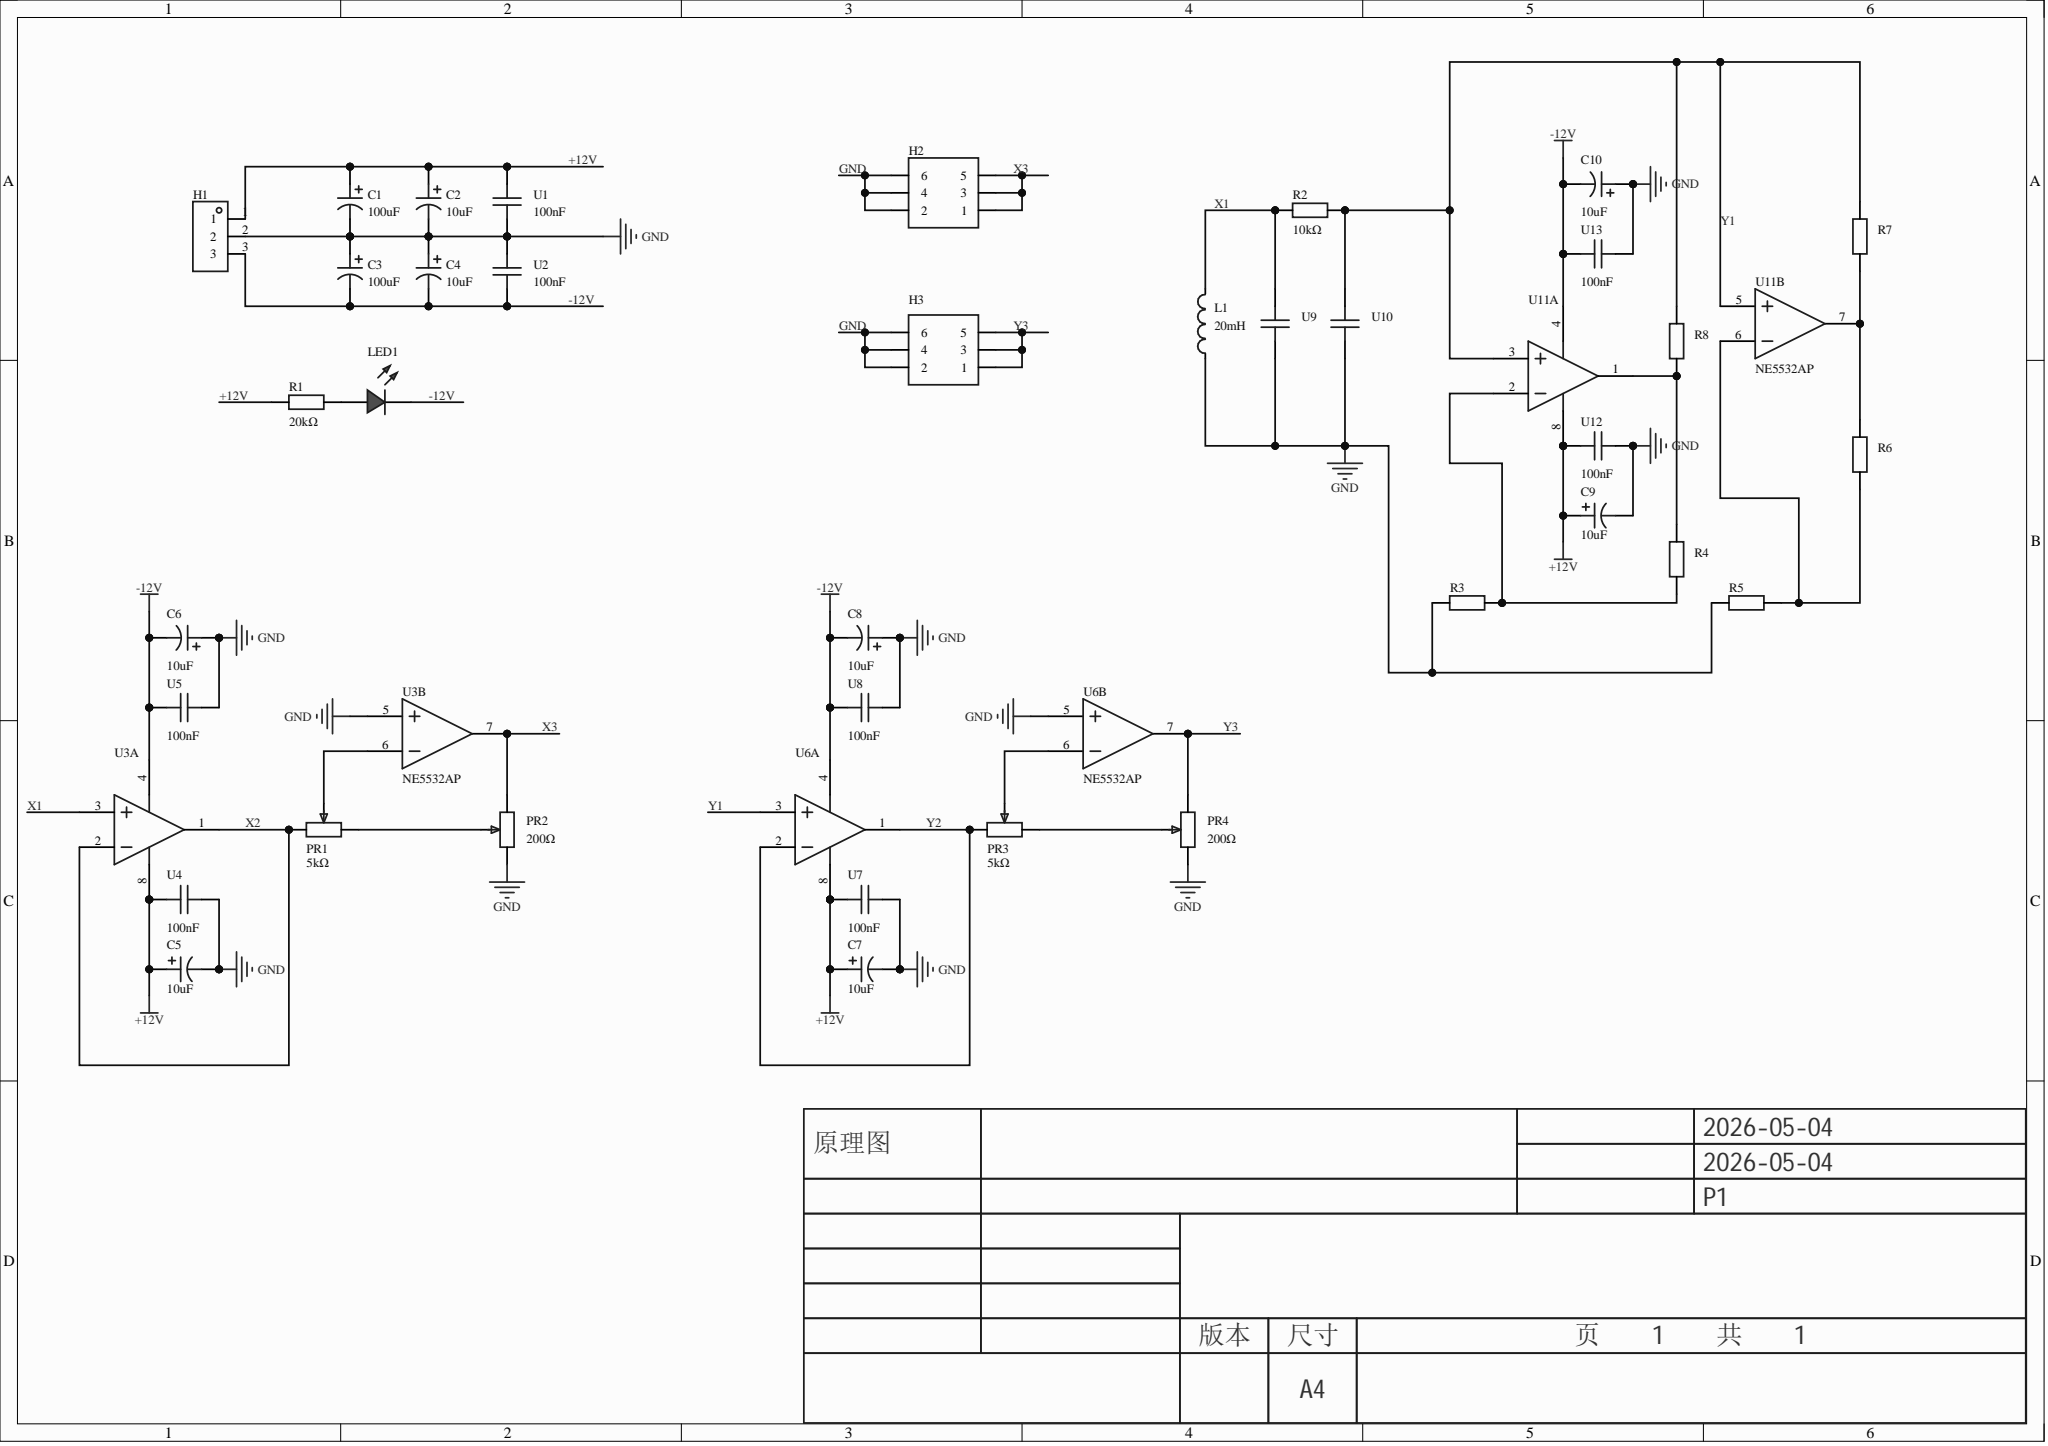Circuit board | Altium Designer | 40 parts | 18 nets
Bill of materials:
Comment,Description,Designator,Footprint,LibRef,Quantity
"100uF","","C1, C3","CAP-TH_BD8.0-P3.50-D0.6-FD_1","100uF","2"
"10uF","","C2, C4, C5, C6, C7, C8, C9, C10","CAP-TH_BD5.0-P2.00-D0.8-FD-10UF50VC110GL","10UF50VC110GL","8"
"","","H1","HDR-TH_3P-P2.54-V-M","HDR-M_2.54_1x3P","1"
"","","H2, H3","HDR-TH_6P-P2.54-V-F-R2-C3-S2.54","HDR-F_2.54_2x3","2"
"20mH","","L1","L0603","L_0603","1"
"","","LED1","LED_TH-3mm","LED_TH-R_3mm","1"
"5kΩ","","PR1, PR3","R_3296","R_3296","2"
"200Ω","","PR2, PR4","R_3296","R_3296","2"
"20kΩ","","R1","Res_1/8W","Res_AXIAL-1/8W","1"
"10kΩ","","R2, R3, R4, R5, R6, R7, R8","Res_1/8W","Res_AXIAL-1/8W","7"
"100nF","","U1, U2, U4, U5, U7, U8, U9, U10, U12, U13","CAP-TH_L5.0-W2.5-P5.00-D1.0","100nF","10"
"NE5532AP","","U3, U6, U11","PDIP-8_L9.6-W6.4-P2.54-LS7.6-BL","NE5532AP","3"
Netlist (Protel format):
[
C1
CAP-TH_BD8.0-P3.50-D0.6-FD_1
100uF



]
[
C2
CAP-TH_BD5.0-P2.00-D0.8-FD-10UF50VC110GL
10uF



]
[
C3
CAP-TH_BD8.0-P3.50-D0.6-FD_1
100uF



]
[
C4
CAP-TH_BD5.0-P2.00-D0.8-FD-10UF50VC110GL
10uF



]
[
C5
CAP-TH_BD5.0-P2.00-D0.8-FD-10UF50VC110GL
10uF



]
[
C6
CAP-TH_BD5.0-P2.00-D0.8-FD-10UF50VC110GL
10uF



]
[
C7
CAP-TH_BD5.0-P2.00-D0.8-FD-10UF50VC110GL
10uF



]
[
C8
CAP-TH_BD5.0-P2.00-D0.8-FD-10UF50VC110GL
10uF



]
[
C9
CAP-TH_BD5.0-P2.00-D0.8-FD-10UF50VC110GL
10uF



]
[
C10
CAP-TH_BD5.0-P2.00-D0.8-FD-10UF50VC110GL
10uF



]
[
H1
HDR-TH_3P-P2.54-V-M




]
[
H2
HDR-TH_6P-P2.54-V-F-R2-C3-S2.54




]
[
H3
HDR-TH_6P-P2.54-V-F-R2-C3-S2.54




]
[
L1
L0603
20mH



]
[
LED1
LED_TH-3mm




]
[
PR1
R_3296
5kΩ



]
[
PR2
R_3296
200Ω



]
[
PR3
R_3296
5kΩ



]
[
PR4
R_3296
200Ω



]
[
R1
Res_1/8W
20kΩ



]
[
R2
Res_1/8W
10kΩ



]
[
R3
Res_1/8W
10kΩ



]
[
R4
Res_1/8W
10kΩ



]
[
R5
Res_1/8W
10kΩ



]
[
R6
Res_1/8W
10kΩ



]
[
R7
Res_1/8W
10kΩ



]
[
R8
Res_1/8W
10kΩ



]
[
U1
CAP-TH_L5.0-W2.5-P5.00-D1.0
100nF



]
[
U2
CAP-TH_L5.0-W2.5-P5.00-D1.0
100nF



]
[
U3
PDIP-8_L9.6-W6.4-P2.54-LS7.6-BL
NE5532AP



]
[
U4
CAP-TH_L5.0-W2.5-P5.00-D1.0
100nF



]
[
U5
CAP-TH_L5.0-W2.5-P5.00-D1.0
100nF



]
[
U6
PDIP-8_L9.6-W6.4-P2.54-LS7.6-BL
NE5532AP



]
[
U7
CAP-TH_L5.0-W2.5-P5.00-D1.0
100nF



]
[
U8
CAP-TH_L5.0-W2.5-P5.00-D1.0
100nF



]
[
U9
CAP-TH_L5.0-W2.5-P5.00-D1.0
100nF



]
[
U10
CAP-TH_L5.0-W2.5-P5.00-D1.0
100nF



]
[
U11
PDIP-8_L9.6-W6.4-P2.54-LS7.6-BL
NE5532AP



]
[
U12
CAP-TH_L5.0-W2.5-P5.00-D1.0
100nF



]
[
U13
CAP-TH_L5.0-W2.5-P5.00-D1.0
100nF



]
(
Y3
H3-1
H3-3
H3-5
PR4-1
U6-7
)
(
Y2
PR3-3
U6-1
U6-2
)
(
Y1
R2-2
R7-2
R8-2
U6-3
U10-1
U11-3
U11-5
)
(
X3
H2-1
H2-3
H2-5
PR2-1
U3-7
)
(
X2
PR1-3
U3-1
U3-2
)
(
X1
L1-2
R2-1
U3-3
U9-1
)
(
NetR6_2
R6-2
R7-1
U11-7
)
(
NetR5_2
R5-2
R6-1
U11-6
)
(
NetR4_2
R4-2
R8-1
U11-1
)
(
NetR3_2
R3-2
R4-1
U11-2
)
(
NetPR3_2
PR3-2
U6-6
)
(
NetPR3_1
PR3-1
PR4-2
)
(
NetPR1_2
PR1-2
U3-6
)
(
NetPR1_1
PR1-1
PR2-2
)
(
NetLED1_1
LED1-1
R1-2
)
(
GND
C1-2
C2-2
C3-1
C4-1
C5-2
C6-1
C7-2
C8-1
C9-2
C10-1
H1-2
H2-2
H2-4
H2-6
H3-2
H3-4
H3-6
L1-1
PR2-3
PR4-3
R3-1
R5-1
U1-2
U2-1
U3-5
U4-1
U5-1
U6-5
U7-1
U8-1
U9-2
U10-2
U12-1
U13-1
)
(
-12V
C3-2
C4-2
C6-2
C8-2
C10-2
H1-3
LED1-2
U2-2
U3-4
U5-2
U6-4
U8-2
U11-4
U13-2
)
(
+12V
C1-1
C2-1
C5-1
C7-1
C9-1
H1-1
R1-1
U1-1
U3-8
U4-2
U6-8
U7-2
U11-8
U12-2
)